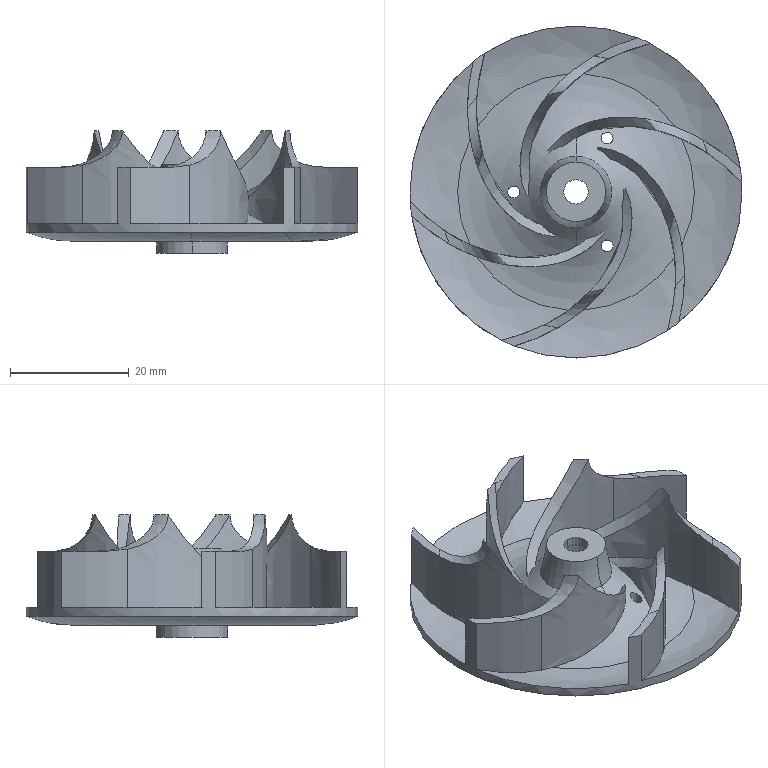Part | STEP file | PRT0001_20_1_1_1 | 1 solid | 83 faces | box 56 x 56 x 20.61 mm | volume 7408 mm3 | other 24 | plane 19 | spline 16 | cylinder 14 | torus 10 | commonest cylinder face diameters 2 x6 4.1 x2 8 x2 12 x2 56 x2